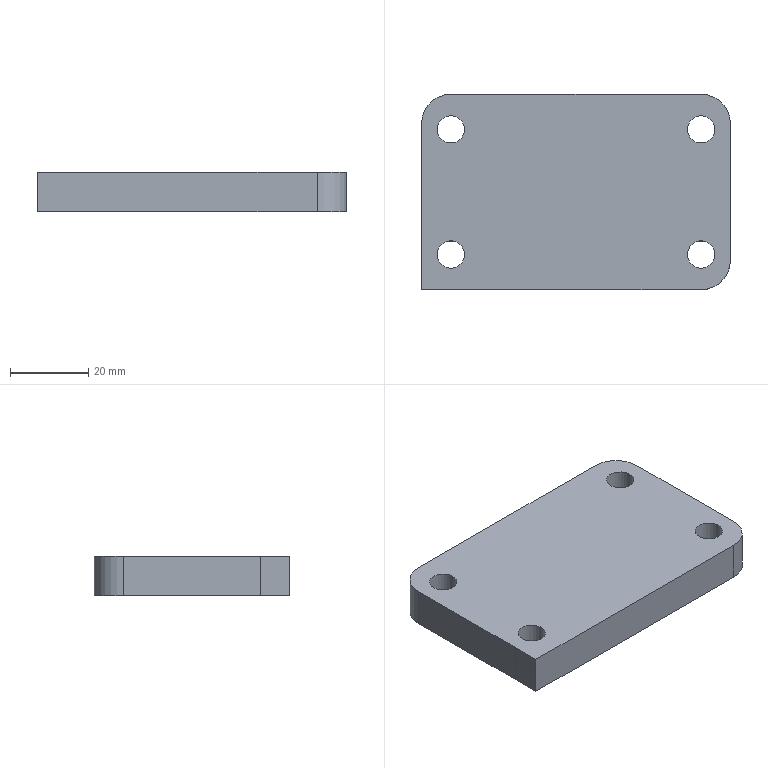Part | NX | features solid 2 | 1 solid | 14 faces | box 79 x 50 x 10 mm | volume 37598 mm3 | plane 7 | cylinder 7 | commonest cylinder face diameters 7 x4 15 x3
STEP:
#1=CARTESIAN_POINT('',(-374.5,452.5,-25.));
#2=VERTEX_POINT('',#1);
#3=CARTESIAN_POINT('',(-374.5,417.5,-25.));
#4=VERTEX_POINT('',#3);
#5=CARTESIAN_POINT('',(-374.5,460.,-25.));
#6=DIRECTION('',(0.,-1.,0.));
#7=VECTOR('',#6,1000.);
#8=LINE('',#5,#7);
#9=EDGE_CURVE('',#2,#4,#8,.T.);
#10=ORIENTED_EDGE('',*,*,#9,.F.);
#11=CARTESIAN_POINT('',(-374.5,452.5,-35.));
#12=VERTEX_POINT('',#11);
#13=CARTESIAN_POINT('',(-374.5,452.5,-25.));
#14=DIRECTION('',(0.,0.,-1.));
#15=VECTOR('',#14,1000.);
#16=LINE('',#13,#15);
#17=EDGE_CURVE('',#12,#2,#16,.F.);
#18=ORIENTED_EDGE('',*,*,#17,.F.);
#19=CARTESIAN_POINT('',(-374.5,417.5,-35.));
#20=VERTEX_POINT('',#19);
#21=CARTESIAN_POINT('',(-374.5,460.,-35.));
#22=DIRECTION('',(0.,-1.,0.));
#23=VECTOR('',#22,1000.);
#24=LINE('',#21,#23);
#25=EDGE_CURVE('',#12,#20,#24,.T.);
#26=ORIENTED_EDGE('',*,*,#25,.T.);
#27=CARTESIAN_POINT('',(-374.5,417.5,-25.));
#28=DIRECTION('',(0.,0.,-1.));
#29=VECTOR('',#28,1000.);
#30=LINE('',#27,#29);
#31=EDGE_CURVE('',#4,#20,#30,.T.);
#32=ORIENTED_EDGE('',*,*,#31,.F.);
#33=EDGE_LOOP('',(#10,#18,#26,#32));
#34=FACE_BOUND('',#33,.T.);
#35=CARTESIAN_POINT('',(-374.5,460.,-25.));
#36=DIRECTION('',(-1.,0.,0.));
#37=DIRECTION('',(0.,1.,0.));
#38=AXIS2_PLACEMENT_3D('',#35,#36,#37);
#39=PLANE('',#38);
#40=ADVANCED_FACE('',(#34),#39,.T.);
#41=CARTESIAN_POINT('',(-374.5,410.,-25.));
#42=VERTEX_POINT('',#41);
#43=CARTESIAN_POINT('',(-303.,410.,-25.));
#44=VERTEX_POINT('',#43);
#45=CARTESIAN_POINT('',(-374.5,410.,-25.));
#46=DIRECTION('',(1.,0.,0.));
#47=VECTOR('',#46,1000.);
#48=LINE('',#45,#47);
#49=EDGE_CURVE('',#42,#44,#48,.T.);
#50=ORIENTED_EDGE('',*,*,#49,.F.);
#51=CARTESIAN_POINT('',(-374.5,410.,-35.));
#52=VERTEX_POINT('',#51);
#53=CARTESIAN_POINT('',(-374.5,410.,-25.));
#54=DIRECTION('',(0.,0.,1.));
#55=VECTOR('',#54,1000.);
#56=LINE('',#53,#55);
#57=EDGE_CURVE('',#52,#42,#56,.T.);
#58=ORIENTED_EDGE('',*,*,#57,.F.);
#59=CARTESIAN_POINT('',(-303.,410.,-35.));
#60=VERTEX_POINT('',#59);
#61=CARTESIAN_POINT('',(-374.5,410.,-35.));
#62=DIRECTION('',(1.,0.,0.));
#63=VECTOR('',#62,1000.);
#64=LINE('',#61,#63);
#65=EDGE_CURVE('',#52,#60,#64,.T.);
#66=ORIENTED_EDGE('',*,*,#65,.T.);
#67=CARTESIAN_POINT('',(-303.,410.,-25.));
#68=DIRECTION('',(0.,0.,-1.));
#69=VECTOR('',#68,1000.);
#70=LINE('',#67,#69);
#71=EDGE_CURVE('',#44,#60,#70,.T.);
#72=ORIENTED_EDGE('',*,*,#71,.F.);
#73=EDGE_LOOP('',(#50,#58,#66,#72));
#74=FACE_BOUND('',#73,.T.);
#75=CARTESIAN_POINT('',(-374.5,410.,-25.));
#76=DIRECTION('',(0.,-1.,0.));
#77=DIRECTION('',(-1.,0.,0.));
#78=AXIS2_PLACEMENT_3D('',#75,#76,#77);
#79=PLANE('',#78);
#80=ADVANCED_FACE('',(#74),#79,.T.);
#81=CARTESIAN_POINT('',(-295.5,417.5,-35.));
#82=VERTEX_POINT('',#81);
#83=CARTESIAN_POINT('',(-295.5,452.5,-35.));
#84=VERTEX_POINT('',#83);
#85=CARTESIAN_POINT('',(-295.5,410.,-35.));
#86=DIRECTION('',(0.,1.,0.));
#87=VECTOR('',#86,1000.);
#88=LINE('',#85,#87);
#89=EDGE_CURVE('',#82,#84,#88,.T.);
#90=ORIENTED_EDGE('',*,*,#89,.T.);
#91=CARTESIAN_POINT('',(-295.5,452.5,-25.));
#92=VERTEX_POINT('',#91);
#93=CARTESIAN_POINT('',(-295.5,452.5,-25.));
#94=DIRECTION('',(0.,0.,-1.));
#95=VECTOR('',#94,1000.);
#96=LINE('',#93,#95);
#97=EDGE_CURVE('',#92,#84,#96,.T.);
#98=ORIENTED_EDGE('',*,*,#97,.F.);
#99=CARTESIAN_POINT('',(-295.5,417.5,-25.));
#100=VERTEX_POINT('',#99);
#101=CARTESIAN_POINT('',(-295.5,410.,-25.));
#102=DIRECTION('',(0.,1.,0.));
#103=VECTOR('',#102,1000.);
#104=LINE('',#101,#103);
#105=EDGE_CURVE('',#100,#92,#104,.T.);
#106=ORIENTED_EDGE('',*,*,#105,.F.);
#107=CARTESIAN_POINT('',(-295.5,417.5,-25.));
#108=DIRECTION('',(0.,0.,-1.));
#109=VECTOR('',#108,1000.);
#110=LINE('',#107,#109);
#111=EDGE_CURVE('',#82,#100,#110,.F.);
#112=ORIENTED_EDGE('',*,*,#111,.F.);
#113=EDGE_LOOP('',(#90,#98,#106,#112));
#114=FACE_BOUND('',#113,.T.);
#115=CARTESIAN_POINT('',(-295.5,410.,-25.));
#116=DIRECTION('',(1.,0.,0.));
#117=DIRECTION('',(0.,-1.,0.));
#118=AXIS2_PLACEMENT_3D('',#115,#116,#117);
#119=PLANE('',#118);
#120=ADVANCED_FACE('',(#114),#119,.T.);
#121=CARTESIAN_POINT('',(-303.,460.,-35.));
#122=VERTEX_POINT('',#121);
#123=CARTESIAN_POINT('',(-367.,460.,-35.));
#124=VERTEX_POINT('',#123);
#125=CARTESIAN_POINT('',(-295.5,460.,-35.));
#126=DIRECTION('',(-1.,0.,0.));
#127=VECTOR('',#126,1000.);
#128=LINE('',#125,#127);
#129=EDGE_CURVE('',#122,#124,#128,.T.);
#130=ORIENTED_EDGE('',*,*,#129,.T.);
#131=CARTESIAN_POINT('',(-367.,460.,-25.));
#132=VERTEX_POINT('',#131);
#133=CARTESIAN_POINT('',(-367.,460.,-25.));
#134=DIRECTION('',(0.,0.,-1.));
#135=VECTOR('',#134,1000.);
#136=LINE('',#133,#135);
#137=EDGE_CURVE('',#132,#124,#136,.T.);
#138=ORIENTED_EDGE('',*,*,#137,.F.);
#139=CARTESIAN_POINT('',(-303.,460.,-25.));
#140=VERTEX_POINT('',#139);
#141=CARTESIAN_POINT('',(-295.5,460.,-25.));
#142=DIRECTION('',(-1.,0.,0.));
#143=VECTOR('',#142,1000.);
#144=LINE('',#141,#143);
#145=EDGE_CURVE('',#140,#132,#144,.T.);
#146=ORIENTED_EDGE('',*,*,#145,.F.);
#147=CARTESIAN_POINT('',(-303.,460.,-25.));
#148=DIRECTION('',(0.,0.,-1.));
#149=VECTOR('',#148,1000.);
#150=LINE('',#147,#149);
#151=EDGE_CURVE('',#122,#140,#150,.F.);
#152=ORIENTED_EDGE('',*,*,#151,.F.);
#153=EDGE_LOOP('',(#130,#138,#146,#152));
#154=FACE_BOUND('',#153,.T.);
#155=CARTESIAN_POINT('',(-295.5,460.,-25.));
#156=DIRECTION('',(0.,1.,0.));
#157=DIRECTION('',(1.,0.,0.));
#158=AXIS2_PLACEMENT_3D('',#155,#156,#157);
#159=PLANE('',#158);
#160=ADVANCED_FACE('',(#154),#159,.T.);
#161=CARTESIAN_POINT('',(-299.5,451.,-25.));
#162=VERTEX_POINT('',#161);
#163=CARTESIAN_POINT('',(-303.,451.,-25.));
#164=DIRECTION('',(0.,0.,1.));
#165=DIRECTION('',(1.,0.,0.));
#166=AXIS2_PLACEMENT_3D('',#163,#164,#165);
#167=CIRCLE('',#166,3.5);
#168=EDGE_CURVE('',#162,#162,#167,.T.);
#169=ORIENTED_EDGE('',*,*,#168,.F.);
#170=EDGE_LOOP('',(#169));
#171=FACE_BOUND('',#170,.T.);
#172=CARTESIAN_POINT('',(-299.5,419.,-25.));
#173=VERTEX_POINT('',#172);
#174=CARTESIAN_POINT('',(-303.,419.,-25.));
#175=DIRECTION('',(0.,0.,-1.));
#176=DIRECTION('',(1.,0.,0.));
#177=AXIS2_PLACEMENT_3D('',#174,#175,#176);
#178=CIRCLE('',#177,3.5);
#179=EDGE_CURVE('',#173,#173,#178,.T.);
#180=ORIENTED_EDGE('',*,*,#179,.T.);
#181=EDGE_LOOP('',(#180));
#182=FACE_BOUND('',#181,.T.);
#183=CARTESIAN_POINT('',(-370.5,451.,-25.));
#184=VERTEX_POINT('',#183);
#185=CARTESIAN_POINT('',(-367.,451.,-25.));
#186=DIRECTION('',(0.,0.,-1.));
#187=DIRECTION('',(-1.,0.,0.));
#188=AXIS2_PLACEMENT_3D('',#185,#186,#187);
#189=CIRCLE('',#188,3.5);
#190=EDGE_CURVE('',#184,#184,#189,.T.);
#191=ORIENTED_EDGE('',*,*,#190,.T.);
#192=EDGE_LOOP('',(#191));
#193=FACE_BOUND('',#192,.T.);
#194=CARTESIAN_POINT('',(-370.5,419.,-25.));
#195=VERTEX_POINT('',#194);
#196=CARTESIAN_POINT('',(-367.,419.,-25.));
#197=DIRECTION('',(0.,0.,1.));
#198=DIRECTION('',(-1.,0.,0.));
#199=AXIS2_PLACEMENT_3D('',#196,#197,#198);
#200=CIRCLE('',#199,3.5);
#201=EDGE_CURVE('',#195,#195,#200,.T.);
#202=ORIENTED_EDGE('',*,*,#201,.F.);
#203=EDGE_LOOP('',(#202));
#204=FACE_BOUND('',#203,.T.);
#205=ORIENTED_EDGE('',*,*,#105,.T.);
#206=CARTESIAN_POINT('',(-303.,452.5,-25.));
#207=DIRECTION('',(0.,0.,-1.));
#208=DIRECTION('',(1.,0.,0.));
#209=AXIS2_PLACEMENT_3D('',#206,#207,#208);
#210=CIRCLE('',#209,7.5);
#211=EDGE_CURVE('',#140,#92,#210,.T.);
#212=ORIENTED_EDGE('',*,*,#211,.F.);
#213=ORIENTED_EDGE('',*,*,#145,.T.);
#214=CARTESIAN_POINT('',(-367.,452.5,-25.));
#215=DIRECTION('',(0.,0.,-1.));
#216=DIRECTION('',(1.,0.,0.));
#217=AXIS2_PLACEMENT_3D('',#214,#215,#216);
#218=CIRCLE('',#217,7.5);
#219=EDGE_CURVE('',#2,#132,#218,.T.);
#220=ORIENTED_EDGE('',*,*,#219,.F.);
#221=ORIENTED_EDGE('',*,*,#9,.T.);
#222=CARTESIAN_POINT('',(-374.5,460.,-25.));
#223=DIRECTION('',(0.,1.,0.));
#224=VECTOR('',#223,1000.);
#225=LINE('',#222,#224);
#226=EDGE_CURVE('',#42,#4,#225,.T.);
#227=ORIENTED_EDGE('',*,*,#226,.F.);
#228=ORIENTED_EDGE('',*,*,#49,.T.);
#229=CARTESIAN_POINT('',(-303.,417.5,-25.));
#230=DIRECTION('',(0.,0.,-1.));
#231=DIRECTION('',(1.,0.,0.));
#232=AXIS2_PLACEMENT_3D('',#229,#230,#231);
#233=CIRCLE('',#232,7.5);
#234=EDGE_CURVE('',#100,#44,#233,.T.);
#235=ORIENTED_EDGE('',*,*,#234,.F.);
#236=EDGE_LOOP('',(#205,#212,#213,#220,#221,#227,#228,#235));
#237=FACE_BOUND('',#236,.T.);
#238=CARTESIAN_POINT('',(-374.5,460.,-25.));
#239=DIRECTION('',(0.,0.,1.));
#240=DIRECTION('',(1.,0.,0.));
#241=AXIS2_PLACEMENT_3D('',#238,#239,#240);
#242=PLANE('',#241);
#243=ADVANCED_FACE('',(#171,#182,#193,#204,#237),#242,.T.);
#244=CARTESIAN_POINT('',(-299.5,451.,-35.));
#245=VERTEX_POINT('',#244);
#246=CARTESIAN_POINT('',(-303.,451.,-35.));
#247=DIRECTION('',(0.,0.,1.));
#248=DIRECTION('',(1.,0.,0.));
#249=AXIS2_PLACEMENT_3D('',#246,#247,#248);
#250=CIRCLE('',#249,3.5);
#251=EDGE_CURVE('',#245,#245,#250,.T.);
#252=ORIENTED_EDGE('',*,*,#251,.T.);
#253=EDGE_LOOP('',(#252));
#254=FACE_BOUND('',#253,.T.);
#255=CARTESIAN_POINT('',(-299.5,419.,-35.));
#256=VERTEX_POINT('',#255);
#257=CARTESIAN_POINT('',(-303.,419.,-35.));
#258=DIRECTION('',(0.,0.,-1.));
#259=DIRECTION('',(1.,0.,0.));
#260=AXIS2_PLACEMENT_3D('',#257,#258,#259);
#261=CIRCLE('',#260,3.5);
#262=EDGE_CURVE('',#256,#256,#261,.T.);
#263=ORIENTED_EDGE('',*,*,#262,.F.);
#264=EDGE_LOOP('',(#263));
#265=FACE_BOUND('',#264,.T.);
#266=CARTESIAN_POINT('',(-370.5,451.,-35.));
#267=VERTEX_POINT('',#266);
#268=CARTESIAN_POINT('',(-367.,451.,-35.));
#269=DIRECTION('',(0.,0.,-1.));
#270=DIRECTION('',(-1.,0.,0.));
#271=AXIS2_PLACEMENT_3D('',#268,#269,#270);
#272=CIRCLE('',#271,3.5);
#273=EDGE_CURVE('',#267,#267,#272,.T.);
#274=ORIENTED_EDGE('',*,*,#273,.F.);
#275=EDGE_LOOP('',(#274));
#276=FACE_BOUND('',#275,.T.);
#277=CARTESIAN_POINT('',(-370.5,419.,-35.));
#278=VERTEX_POINT('',#277);
#279=CARTESIAN_POINT('',(-367.,419.,-35.));
#280=DIRECTION('',(0.,0.,1.));
#281=DIRECTION('',(-1.,0.,0.));
#282=AXIS2_PLACEMENT_3D('',#279,#280,#281);
#283=CIRCLE('',#282,3.5);
#284=EDGE_CURVE('',#278,#278,#283,.T.);
#285=ORIENTED_EDGE('',*,*,#284,.T.);
#286=EDGE_LOOP('',(#285));
#287=FACE_BOUND('',#286,.T.);
#288=ORIENTED_EDGE('',*,*,#65,.F.);
#289=CARTESIAN_POINT('',(-374.5,460.,-35.));
#290=DIRECTION('',(0.,-1.,0.));
#291=VECTOR('',#290,1000.);
#292=LINE('',#289,#291);
#293=EDGE_CURVE('',#20,#52,#292,.T.);
#294=ORIENTED_EDGE('',*,*,#293,.F.);
#295=ORIENTED_EDGE('',*,*,#25,.F.);
#296=CARTESIAN_POINT('',(-367.,452.5,-35.));
#297=DIRECTION('',(0.,0.,-1.));
#298=DIRECTION('',(1.,0.,0.));
#299=AXIS2_PLACEMENT_3D('',#296,#297,#298);
#300=CIRCLE('',#299,7.5);
#301=EDGE_CURVE('',#124,#12,#300,.F.);
#302=ORIENTED_EDGE('',*,*,#301,.F.);
#303=ORIENTED_EDGE('',*,*,#129,.F.);
#304=CARTESIAN_POINT('',(-303.,452.5,-35.));
#305=DIRECTION('',(0.,0.,-1.));
#306=DIRECTION('',(1.,0.,0.));
#307=AXIS2_PLACEMENT_3D('',#304,#305,#306);
#308=CIRCLE('',#307,7.5);
#309=EDGE_CURVE('',#84,#122,#308,.F.);
#310=ORIENTED_EDGE('',*,*,#309,.F.);
#311=ORIENTED_EDGE('',*,*,#89,.F.);
#312=CARTESIAN_POINT('',(-303.,417.5,-35.));
#313=DIRECTION('',(0.,0.,-1.));
#314=DIRECTION('',(1.,0.,0.));
#315=AXIS2_PLACEMENT_3D('',#312,#313,#314);
#316=CIRCLE('',#315,7.5);
#317=EDGE_CURVE('',#60,#82,#316,.F.);
#318=ORIENTED_EDGE('',*,*,#317,.F.);
#319=EDGE_LOOP('',(#288,#294,#295,#302,#303,#310,#311,#318));
#320=FACE_BOUND('',#319,.T.);
#321=CARTESIAN_POINT('',(-374.5,460.,-35.));
#322=DIRECTION('',(0.,0.,1.));
#323=DIRECTION('',(1.,0.,0.));
#324=AXIS2_PLACEMENT_3D('',#321,#322,#323);
#325=PLANE('',#324);
#326=ADVANCED_FACE('',(#254,#265,#276,#287,#320),#325,.F.);
#327=ORIENTED_EDGE('',*,*,#234,.T.);
#328=ORIENTED_EDGE('',*,*,#71,.T.);
#329=ORIENTED_EDGE('',*,*,#317,.T.);
#330=ORIENTED_EDGE('',*,*,#111,.T.);
#331=EDGE_LOOP('',(#327,#328,#329,#330));
#332=FACE_BOUND('',#331,.T.);
#333=CARTESIAN_POINT('',(-303.,417.5,-25.));
#334=DIRECTION('',(0.,0.,-1.));
#335=DIRECTION('',(-1.,0.,0.));
#336=AXIS2_PLACEMENT_3D('',#333,#334,#335);
#337=CYLINDRICAL_SURFACE('',#336,7.5);
#338=ADVANCED_FACE('',(#332),#337,.T.);
#339=ORIENTED_EDGE('',*,*,#211,.T.);
#340=ORIENTED_EDGE('',*,*,#97,.T.);
#341=ORIENTED_EDGE('',*,*,#309,.T.);
#342=ORIENTED_EDGE('',*,*,#151,.T.);
#343=EDGE_LOOP('',(#339,#340,#341,#342));
#344=FACE_BOUND('',#343,.T.);
#345=CARTESIAN_POINT('',(-303.,452.5,-25.));
#346=DIRECTION('',(0.,0.,-1.));
#347=DIRECTION('',(-1.,0.,0.));
#348=AXIS2_PLACEMENT_3D('',#345,#346,#347);
#349=CYLINDRICAL_SURFACE('',#348,7.5);
#350=ADVANCED_FACE('',(#344),#349,.T.);
#351=ORIENTED_EDGE('',*,*,#226,.T.);
#352=ORIENTED_EDGE('',*,*,#31,.T.);
#353=ORIENTED_EDGE('',*,*,#293,.T.);
#354=ORIENTED_EDGE('',*,*,#57,.T.);
#355=EDGE_LOOP('',(#351,#352,#353,#354));
#356=FACE_BOUND('',#355,.T.);
#357=CARTESIAN_POINT('',(-374.5,460.,-25.));
#358=DIRECTION('',(-1.,0.,0.));
#359=DIRECTION('',(0.,1.,0.));
#360=AXIS2_PLACEMENT_3D('',#357,#358,#359);
#361=PLANE('',#360);
#362=ADVANCED_FACE('',(#356),#361,.T.);
#363=ORIENTED_EDGE('',*,*,#219,.T.);
#364=ORIENTED_EDGE('',*,*,#137,.T.);
#365=ORIENTED_EDGE('',*,*,#301,.T.);
#366=ORIENTED_EDGE('',*,*,#17,.T.);
#367=EDGE_LOOP('',(#363,#364,#365,#366));
#368=FACE_BOUND('',#367,.T.);
#369=CARTESIAN_POINT('',(-367.,452.5,-25.));
#370=DIRECTION('',(0.,0.,-1.));
#371=DIRECTION('',(-1.,0.,0.));
#372=AXIS2_PLACEMENT_3D('',#369,#370,#371);
#373=CYLINDRICAL_SURFACE('',#372,7.5);
#374=ADVANCED_FACE('',(#368),#373,.T.);
#375=ORIENTED_EDGE('',*,*,#284,.F.);
#376=EDGE_LOOP('',(#375));
#377=FACE_BOUND('',#376,.T.);
#378=ORIENTED_EDGE('',*,*,#201,.T.);
#379=EDGE_LOOP('',(#378));
#380=FACE_BOUND('',#379,.T.);
#381=CARTESIAN_POINT('',(-367.,419.,-25.));
#382=DIRECTION('',(0.,0.,-1.));
#383=DIRECTION('',(-1.,0.,0.));
#384=AXIS2_PLACEMENT_3D('',#381,#382,#383);
#385=CYLINDRICAL_SURFACE('',#384,3.5);
#386=ADVANCED_FACE('',(#377,#380),#385,.F.);
#387=ORIENTED_EDGE('',*,*,#273,.T.);
#388=EDGE_LOOP('',(#387));
#389=FACE_BOUND('',#388,.T.);
#390=ORIENTED_EDGE('',*,*,#190,.F.);
#391=EDGE_LOOP('',(#390));
#392=FACE_BOUND('',#391,.T.);
#393=CARTESIAN_POINT('',(-367.,451.,-25.));
#394=DIRECTION('',(0.,0.,-1.));
#395=DIRECTION('',(-1.,0.,0.));
#396=AXIS2_PLACEMENT_3D('',#393,#394,#395);
#397=CYLINDRICAL_SURFACE('',#396,3.5);
#398=ADVANCED_FACE('',(#389,#392),#397,.F.);
#399=ORIENTED_EDGE('',*,*,#262,.T.);
#400=EDGE_LOOP('',(#399));
#401=FACE_BOUND('',#400,.T.);
#402=ORIENTED_EDGE('',*,*,#179,.F.);
#403=EDGE_LOOP('',(#402));
#404=FACE_BOUND('',#403,.T.);
#405=CARTESIAN_POINT('',(-303.,419.,-25.));
#406=DIRECTION('',(0.,0.,-1.));
#407=DIRECTION('',(1.,0.,0.));
#408=AXIS2_PLACEMENT_3D('',#405,#406,#407);
#409=CYLINDRICAL_SURFACE('',#408,3.5);
#410=ADVANCED_FACE('',(#401,#404),#409,.F.);
#411=ORIENTED_EDGE('',*,*,#251,.F.);
#412=EDGE_LOOP('',(#411));
#413=FACE_BOUND('',#412,.T.);
#414=ORIENTED_EDGE('',*,*,#168,.T.);
#415=EDGE_LOOP('',(#414));
#416=FACE_BOUND('',#415,.T.);
#417=CARTESIAN_POINT('',(-303.,451.,-25.));
#418=DIRECTION('',(0.,0.,-1.));
#419=DIRECTION('',(1.,0.,0.));
#420=AXIS2_PLACEMENT_3D('',#417,#418,#419);
#421=CYLINDRICAL_SURFACE('',#420,3.5);
#422=ADVANCED_FACE('',(#413,#416),#421,.F.);
#423=CLOSED_SHELL('',(#40,#80,#120,#160,#243,#326,#338,#350,#362,#374,#386,#398,#410,#422));
#424=MANIFOLD_SOLID_BREP('',#423);
#425=(LENGTH_UNIT()NAMED_UNIT(*)SI_UNIT(.MILLI.,.METRE.));
#426=UNCERTAINTY_MEASURE_WITH_UNIT(LENGTH_MEASURE(0.00001),#425,'','');
#427=(NAMED_UNIT(*)PLANE_ANGLE_UNIT()SI_UNIT($,.RADIAN.));
#428=(NAMED_UNIT(*)SI_UNIT($,.STERADIAN.)SOLID_ANGLE_UNIT());
#429=(GEOMETRIC_REPRESENTATION_CONTEXT(3)GLOBAL_UNCERTAINTY_ASSIGNED_CONTEXT((#426))GLOBAL_UNIT_ASSIGNED_CONTEXT((#425,#427,#428))REPRESENTATION_CONTEXT('',''));
#430=ADVANCED_BREP_SHAPE_REPRESENTATION('',(#424),#429);